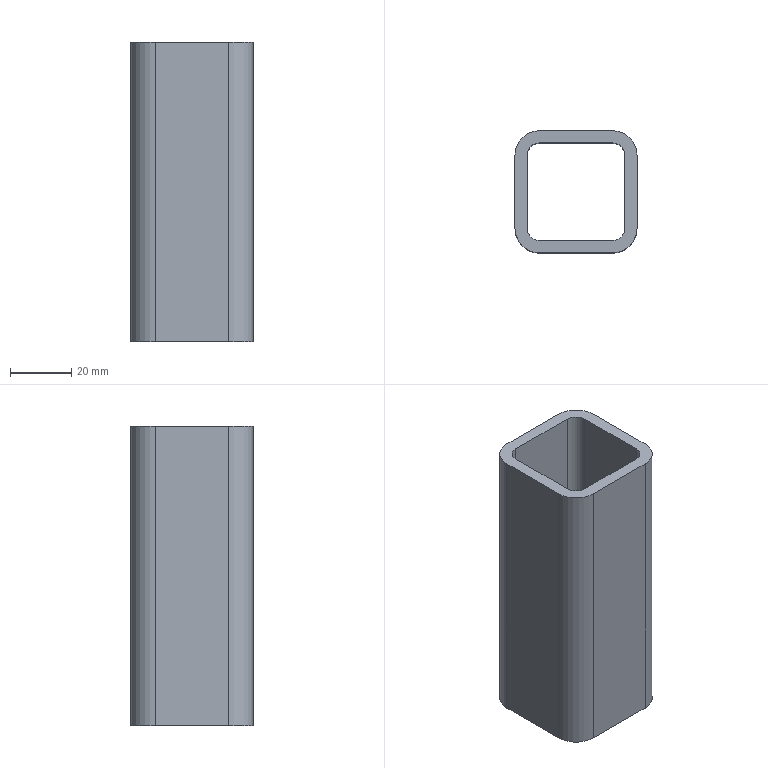Part | STEP file | 40 x 40 x 200 | 1 solid | 18 faces | box 40 x 40 x 98 mm | volume 52410 mm3 | plane 10 | cylinder 8 | commonest cylinder face diameters 8 x4 16 x4
STEP:
#1=CARTESIAN_POINT('',(36.,32.,-502.));
#2=VERTEX_POINT('',#1);
#3=CARTESIAN_POINT('',(32.,36.,-502.));
#4=VERTEX_POINT('',#3);
#5=CARTESIAN_POINT('',(32.,32.,-502.));
#6=DIRECTION('',(0.,0.,1.));
#7=DIRECTION('',(1.,0.,0.));
#8=AXIS2_PLACEMENT_3D('',#5,#6,#7);
#9=CIRCLE('',#8,4.);
#10=EDGE_CURVE('',#2,#4,#9,.T.);
#11=ORIENTED_EDGE('',*,*,#10,.T.);
#12=CARTESIAN_POINT('',(32.,36.,-600.));
#13=VERTEX_POINT('',#12);
#14=CARTESIAN_POINT('',(32.,36.,600.));
#15=DIRECTION('',(0.,0.,1.));
#16=VECTOR('',#15,1000.);
#17=LINE('',#14,#16);
#18=EDGE_CURVE('',#13,#4,#17,.T.);
#19=ORIENTED_EDGE('',*,*,#18,.F.);
#20=CARTESIAN_POINT('',(36.,32.,-600.));
#21=VERTEX_POINT('',#20);
#22=CARTESIAN_POINT('',(32.,32.,-600.));
#23=DIRECTION('',(0.,0.,-1.));
#24=DIRECTION('',(-1.,0.,0.));
#25=AXIS2_PLACEMENT_3D('',#22,#23,#24);
#26=CIRCLE('',#25,4.);
#27=EDGE_CURVE('',#13,#21,#26,.T.);
#28=ORIENTED_EDGE('',*,*,#27,.T.);
#29=CARTESIAN_POINT('',(36.,32.,600.));
#30=DIRECTION('',(0.,0.,-1.));
#31=VECTOR('',#30,1000.);
#32=LINE('',#29,#31);
#33=EDGE_CURVE('',#2,#21,#32,.T.);
#34=ORIENTED_EDGE('',*,*,#33,.F.);
#35=EDGE_LOOP('',(#11,#19,#28,#34));
#36=FACE_OUTER_BOUND('',#35,.T.);
#37=CARTESIAN_POINT('',(32.,32.,600.));
#38=DIRECTION('',(0.,0.,-1.));
#39=DIRECTION('',(-1.,0.,0.));
#40=AXIS2_PLACEMENT_3D('',#37,#38,#39);
#41=CYLINDRICAL_SURFACE('',#40,4.);
#42=ADVANCED_FACE('',(#36),#41,.F.);
#43=CARTESIAN_POINT('',(36.,8.,-600.));
#44=VERTEX_POINT('',#43);
#45=CARTESIAN_POINT('',(36.,8.,-502.));
#46=VERTEX_POINT('',#45);
#47=CARTESIAN_POINT('',(36.,8.,600.));
#48=DIRECTION('',(0.,0.,1.));
#49=VECTOR('',#48,1000.);
#50=LINE('',#47,#49);
#51=EDGE_CURVE('',#44,#46,#50,.T.);
#52=ORIENTED_EDGE('',*,*,#51,.T.);
#53=CARTESIAN_POINT('',(36.,32.,-502.));
#54=DIRECTION('',(0.,1.,0.));
#55=VECTOR('',#54,1000.);
#56=LINE('',#53,#55);
#57=EDGE_CURVE('',#46,#2,#56,.T.);
#58=ORIENTED_EDGE('',*,*,#57,.T.);
#59=ORIENTED_EDGE('',*,*,#33,.T.);
#60=CARTESIAN_POINT('',(36.,32.,-600.));
#61=DIRECTION('',(0.,-1.,0.));
#62=VECTOR('',#61,1000.);
#63=LINE('',#60,#62);
#64=EDGE_CURVE('',#21,#44,#63,.T.);
#65=ORIENTED_EDGE('',*,*,#64,.T.);
#66=EDGE_LOOP('',(#52,#58,#59,#65));
#67=FACE_OUTER_BOUND('',#66,.T.);
#68=CARTESIAN_POINT('',(36.,32.,600.));
#69=DIRECTION('',(-1.,0.,0.));
#70=DIRECTION('',(0.,0.,1.));
#71=AXIS2_PLACEMENT_3D('',#68,#69,#70);
#72=PLANE('',#71);
#73=ADVANCED_FACE('',(#67),#72,.T.);
#74=CARTESIAN_POINT('',(32.,4.,-502.));
#75=VERTEX_POINT('',#74);
#76=CARTESIAN_POINT('',(32.,8.,-502.));
#77=DIRECTION('',(0.,0.,1.));
#78=DIRECTION('',(1.,0.,0.));
#79=AXIS2_PLACEMENT_3D('',#76,#77,#78);
#80=CIRCLE('',#79,4.);
#81=EDGE_CURVE('',#75,#46,#80,.T.);
#82=ORIENTED_EDGE('',*,*,#81,.T.);
#83=ORIENTED_EDGE('',*,*,#51,.F.);
#84=CARTESIAN_POINT('',(32.,4.,-600.));
#85=VERTEX_POINT('',#84);
#86=CARTESIAN_POINT('',(32.,8.,-600.));
#87=DIRECTION('',(0.,0.,-1.));
#88=DIRECTION('',(-1.,0.,0.));
#89=AXIS2_PLACEMENT_3D('',#86,#87,#88);
#90=CIRCLE('',#89,4.);
#91=EDGE_CURVE('',#44,#85,#90,.T.);
#92=ORIENTED_EDGE('',*,*,#91,.T.);
#93=CARTESIAN_POINT('',(32.,4.,600.));
#94=DIRECTION('',(0.,0.,-1.));
#95=VECTOR('',#94,1000.);
#96=LINE('',#93,#95);
#97=EDGE_CURVE('',#75,#85,#96,.T.);
#98=ORIENTED_EDGE('',*,*,#97,.F.);
#99=EDGE_LOOP('',(#82,#83,#92,#98));
#100=FACE_OUTER_BOUND('',#99,.T.);
#101=CARTESIAN_POINT('',(32.,8.,600.));
#102=DIRECTION('',(0.,0.,-1.));
#103=DIRECTION('',(-1.,0.,0.));
#104=AXIS2_PLACEMENT_3D('',#101,#102,#103);
#105=CYLINDRICAL_SURFACE('',#104,4.);
#106=ADVANCED_FACE('',(#100),#105,.F.);
#107=CARTESIAN_POINT('',(8.,4.,-600.));
#108=VERTEX_POINT('',#107);
#109=CARTESIAN_POINT('',(8.,4.,-502.));
#110=VERTEX_POINT('',#109);
#111=CARTESIAN_POINT('',(8.,4.,600.));
#112=DIRECTION('',(0.,0.,1.));
#113=VECTOR('',#112,1000.);
#114=LINE('',#111,#113);
#115=EDGE_CURVE('',#108,#110,#114,.T.);
#116=ORIENTED_EDGE('',*,*,#115,.T.);
#117=CARTESIAN_POINT('',(32.,4.,-502.));
#118=DIRECTION('',(1.,0.,0.));
#119=VECTOR('',#118,1000.);
#120=LINE('',#117,#119);
#121=EDGE_CURVE('',#110,#75,#120,.T.);
#122=ORIENTED_EDGE('',*,*,#121,.T.);
#123=ORIENTED_EDGE('',*,*,#97,.T.);
#124=CARTESIAN_POINT('',(32.,4.,-600.));
#125=DIRECTION('',(-1.,0.,0.));
#126=VECTOR('',#125,1000.);
#127=LINE('',#124,#126);
#128=EDGE_CURVE('',#85,#108,#127,.T.);
#129=ORIENTED_EDGE('',*,*,#128,.T.);
#130=EDGE_LOOP('',(#116,#122,#123,#129));
#131=FACE_OUTER_BOUND('',#130,.T.);
#132=CARTESIAN_POINT('',(8.,4.,600.));
#133=DIRECTION('',(0.,1.,0.));
#134=DIRECTION('',(-1.,0.,0.));
#135=AXIS2_PLACEMENT_3D('',#132,#133,#134);
#136=PLANE('',#135);
#137=ADVANCED_FACE('',(#131),#136,.T.);
#138=CARTESIAN_POINT('',(4.,8.,-502.));
#139=VERTEX_POINT('',#138);
#140=CARTESIAN_POINT('',(8.,8.,-502.));
#141=DIRECTION('',(0.,0.,1.));
#142=DIRECTION('',(1.,0.,0.));
#143=AXIS2_PLACEMENT_3D('',#140,#141,#142);
#144=CIRCLE('',#143,4.);
#145=EDGE_CURVE('',#139,#110,#144,.T.);
#146=ORIENTED_EDGE('',*,*,#145,.T.);
#147=ORIENTED_EDGE('',*,*,#115,.F.);
#148=CARTESIAN_POINT('',(4.,8.,-600.));
#149=VERTEX_POINT('',#148);
#150=CARTESIAN_POINT('',(8.,8.,-600.));
#151=DIRECTION('',(0.,0.,-1.));
#152=DIRECTION('',(-1.,0.,0.));
#153=AXIS2_PLACEMENT_3D('',#150,#151,#152);
#154=CIRCLE('',#153,4.);
#155=EDGE_CURVE('',#108,#149,#154,.T.);
#156=ORIENTED_EDGE('',*,*,#155,.T.);
#157=CARTESIAN_POINT('',(4.,8.,600.));
#158=DIRECTION('',(0.,0.,-1.));
#159=VECTOR('',#158,1000.);
#160=LINE('',#157,#159);
#161=EDGE_CURVE('',#139,#149,#160,.T.);
#162=ORIENTED_EDGE('',*,*,#161,.F.);
#163=EDGE_LOOP('',(#146,#147,#156,#162));
#164=FACE_OUTER_BOUND('',#163,.T.);
#165=CARTESIAN_POINT('',(8.,8.,600.));
#166=DIRECTION('',(0.,0.,-1.));
#167=DIRECTION('',(-1.,0.,0.));
#168=AXIS2_PLACEMENT_3D('',#165,#166,#167);
#169=CYLINDRICAL_SURFACE('',#168,4.);
#170=ADVANCED_FACE('',(#164),#169,.F.);
#171=CARTESIAN_POINT('',(4.,32.,-600.));
#172=VERTEX_POINT('',#171);
#173=CARTESIAN_POINT('',(4.,32.,-502.));
#174=VERTEX_POINT('',#173);
#175=CARTESIAN_POINT('',(4.,32.,600.));
#176=DIRECTION('',(0.,0.,1.));
#177=VECTOR('',#176,1000.);
#178=LINE('',#175,#177);
#179=EDGE_CURVE('',#172,#174,#178,.T.);
#180=ORIENTED_EDGE('',*,*,#179,.T.);
#181=CARTESIAN_POINT('',(4.,8.,-502.));
#182=DIRECTION('',(0.,-1.,0.));
#183=VECTOR('',#182,1000.);
#184=LINE('',#181,#183);
#185=EDGE_CURVE('',#174,#139,#184,.T.);
#186=ORIENTED_EDGE('',*,*,#185,.T.);
#187=ORIENTED_EDGE('',*,*,#161,.T.);
#188=CARTESIAN_POINT('',(4.,32.,-600.));
#189=DIRECTION('',(0.,1.,0.));
#190=VECTOR('',#189,1000.);
#191=LINE('',#188,#190);
#192=EDGE_CURVE('',#149,#172,#191,.T.);
#193=ORIENTED_EDGE('',*,*,#192,.T.);
#194=EDGE_LOOP('',(#180,#186,#187,#193));
#195=FACE_OUTER_BOUND('',#194,.T.);
#196=CARTESIAN_POINT('',(4.,8.,600.));
#197=DIRECTION('',(1.,0.,0.));
#198=DIRECTION('',(0.,1.,0.));
#199=AXIS2_PLACEMENT_3D('',#196,#197,#198);
#200=PLANE('',#199);
#201=ADVANCED_FACE('',(#195),#200,.T.);
#202=CARTESIAN_POINT('',(8.,36.,-502.));
#203=VERTEX_POINT('',#202);
#204=CARTESIAN_POINT('',(8.,32.,-502.));
#205=DIRECTION('',(0.,0.,1.));
#206=DIRECTION('',(1.,0.,0.));
#207=AXIS2_PLACEMENT_3D('',#204,#205,#206);
#208=CIRCLE('',#207,4.);
#209=EDGE_CURVE('',#203,#174,#208,.T.);
#210=ORIENTED_EDGE('',*,*,#209,.T.);
#211=ORIENTED_EDGE('',*,*,#179,.F.);
#212=CARTESIAN_POINT('',(8.,36.,-600.));
#213=VERTEX_POINT('',#212);
#214=CARTESIAN_POINT('',(8.,32.,-600.));
#215=DIRECTION('',(0.,0.,-1.));
#216=DIRECTION('',(-1.,0.,0.));
#217=AXIS2_PLACEMENT_3D('',#214,#215,#216);
#218=CIRCLE('',#217,4.);
#219=EDGE_CURVE('',#172,#213,#218,.T.);
#220=ORIENTED_EDGE('',*,*,#219,.T.);
#221=CARTESIAN_POINT('',(8.,36.,600.));
#222=DIRECTION('',(0.,0.,-1.));
#223=VECTOR('',#222,1000.);
#224=LINE('',#221,#223);
#225=EDGE_CURVE('',#203,#213,#224,.T.);
#226=ORIENTED_EDGE('',*,*,#225,.F.);
#227=EDGE_LOOP('',(#210,#211,#220,#226));
#228=FACE_OUTER_BOUND('',#227,.T.);
#229=CARTESIAN_POINT('',(8.,32.,600.));
#230=DIRECTION('',(0.,0.,-1.));
#231=DIRECTION('',(-1.,0.,0.));
#232=AXIS2_PLACEMENT_3D('',#229,#230,#231);
#233=CYLINDRICAL_SURFACE('',#232,4.);
#234=ADVANCED_FACE('',(#228),#233,.F.);
#235=ORIENTED_EDGE('',*,*,#18,.T.);
#236=CARTESIAN_POINT('',(8.,36.,-502.));
#237=DIRECTION('',(-1.,0.,0.));
#238=VECTOR('',#237,1000.);
#239=LINE('',#236,#238);
#240=EDGE_CURVE('',#4,#203,#239,.T.);
#241=ORIENTED_EDGE('',*,*,#240,.T.);
#242=ORIENTED_EDGE('',*,*,#225,.T.);
#243=CARTESIAN_POINT('',(32.,36.,-600.));
#244=DIRECTION('',(1.,0.,0.));
#245=VECTOR('',#244,1000.);
#246=LINE('',#243,#245);
#247=EDGE_CURVE('',#213,#13,#246,.T.);
#248=ORIENTED_EDGE('',*,*,#247,.T.);
#249=EDGE_LOOP('',(#235,#241,#242,#248));
#250=FACE_OUTER_BOUND('',#249,.T.);
#251=CARTESIAN_POINT('',(32.,36.,600.));
#252=DIRECTION('',(0.,-1.,0.));
#253=DIRECTION('',(0.,0.,-1.));
#254=AXIS2_PLACEMENT_3D('',#251,#252,#253);
#255=PLANE('',#254);
#256=ADVANCED_FACE('',(#250),#255,.T.);
#257=CARTESIAN_POINT('',(40.,8.,-600.));
#258=VERTEX_POINT('',#257);
#259=CARTESIAN_POINT('',(40.,8.,-502.));
#260=VERTEX_POINT('',#259);
#261=CARTESIAN_POINT('',(40.,8.,600.));
#262=DIRECTION('',(0.,0.,1.));
#263=VECTOR('',#262,1000.);
#264=LINE('',#261,#263);
#265=EDGE_CURVE('',#258,#260,#264,.T.);
#266=ORIENTED_EDGE('',*,*,#265,.T.);
#267=CARTESIAN_POINT('',(32.,0.,-502.));
#268=VERTEX_POINT('',#267);
#269=CARTESIAN_POINT('',(32.,8.,-502.));
#270=DIRECTION('',(0.,0.,1.));
#271=DIRECTION('',(1.,0.,0.));
#272=AXIS2_PLACEMENT_3D('',#269,#270,#271);
#273=CIRCLE('',#272,8.);
#274=EDGE_CURVE('',#268,#260,#273,.T.);
#275=ORIENTED_EDGE('',*,*,#274,.F.);
#276=CARTESIAN_POINT('',(32.,0.,-600.));
#277=VERTEX_POINT('',#276);
#278=CARTESIAN_POINT('',(32.,0.,600.));
#279=DIRECTION('',(0.,0.,-1.));
#280=VECTOR('',#279,1000.);
#281=LINE('',#278,#280);
#282=EDGE_CURVE('',#268,#277,#281,.T.);
#283=ORIENTED_EDGE('',*,*,#282,.T.);
#284=CARTESIAN_POINT('',(32.,8.,-600.));
#285=DIRECTION('',(0.,0.,1.));
#286=DIRECTION('',(-1.,0.,0.));
#287=AXIS2_PLACEMENT_3D('',#284,#285,#286);
#288=CIRCLE('',#287,8.);
#289=EDGE_CURVE('',#277,#258,#288,.T.);
#290=ORIENTED_EDGE('',*,*,#289,.T.);
#291=EDGE_LOOP('',(#266,#275,#283,#290));
#292=FACE_OUTER_BOUND('',#291,.T.);
#293=CARTESIAN_POINT('',(32.,8.,600.));
#294=DIRECTION('',(0.,0.,-1.));
#295=DIRECTION('',(-1.,0.,0.));
#296=AXIS2_PLACEMENT_3D('',#293,#294,#295);
#297=CYLINDRICAL_SURFACE('',#296,8.);
#298=ADVANCED_FACE('',(#292),#297,.T.);
#299=CARTESIAN_POINT('',(40.,32.,-502.));
#300=VERTEX_POINT('',#299);
#301=CARTESIAN_POINT('',(40.,8.,-502.));
#302=DIRECTION('',(0.,1.,0.));
#303=VECTOR('',#302,1000.);
#304=LINE('',#301,#303);
#305=EDGE_CURVE('',#260,#300,#304,.T.);
#306=ORIENTED_EDGE('',*,*,#305,.F.);
#307=ORIENTED_EDGE('',*,*,#265,.F.);
#308=CARTESIAN_POINT('',(40.,32.,-600.));
#309=VERTEX_POINT('',#308);
#310=CARTESIAN_POINT('',(40.,32.,-600.));
#311=DIRECTION('',(0.,1.,0.));
#312=VECTOR('',#311,1000.);
#313=LINE('',#310,#312);
#314=EDGE_CURVE('',#258,#309,#313,.T.);
#315=ORIENTED_EDGE('',*,*,#314,.T.);
#316=CARTESIAN_POINT('',(40.,32.,600.));
#317=DIRECTION('',(0.,0.,-1.));
#318=VECTOR('',#317,1000.);
#319=LINE('',#316,#318);
#320=EDGE_CURVE('',#300,#309,#319,.T.);
#321=ORIENTED_EDGE('',*,*,#320,.F.);
#322=EDGE_LOOP('',(#306,#307,#315,#321));
#323=FACE_OUTER_BOUND('',#322,.T.);
#324=CARTESIAN_POINT('',(40.,32.,600.));
#325=DIRECTION('',(-1.,0.,0.));
#326=DIRECTION('',(0.,-1.,0.));
#327=AXIS2_PLACEMENT_3D('',#324,#325,#326);
#328=PLANE('',#327);
#329=ADVANCED_FACE('',(#323),#328,.F.);
#330=CARTESIAN_POINT('',(32.,40.,-600.));
#331=VERTEX_POINT('',#330);
#332=CARTESIAN_POINT('',(32.,40.,-502.));
#333=VERTEX_POINT('',#332);
#334=CARTESIAN_POINT('',(32.,40.,600.));
#335=DIRECTION('',(0.,0.,1.));
#336=VECTOR('',#335,1000.);
#337=LINE('',#334,#336);
#338=EDGE_CURVE('',#331,#333,#337,.T.);
#339=ORIENTED_EDGE('',*,*,#338,.T.);
#340=CARTESIAN_POINT('',(32.,32.,-502.));
#341=DIRECTION('',(0.,0.,1.));
#342=DIRECTION('',(1.,0.,0.));
#343=AXIS2_PLACEMENT_3D('',#340,#341,#342);
#344=CIRCLE('',#343,8.);
#345=EDGE_CURVE('',#300,#333,#344,.T.);
#346=ORIENTED_EDGE('',*,*,#345,.F.);
#347=ORIENTED_EDGE('',*,*,#320,.T.);
#348=CARTESIAN_POINT('',(32.,32.,-600.));
#349=DIRECTION('',(0.,0.,1.));
#350=DIRECTION('',(-1.,0.,0.));
#351=AXIS2_PLACEMENT_3D('',#348,#349,#350);
#352=CIRCLE('',#351,8.);
#353=EDGE_CURVE('',#309,#331,#352,.T.);
#354=ORIENTED_EDGE('',*,*,#353,.T.);
#355=EDGE_LOOP('',(#339,#346,#347,#354));
#356=FACE_OUTER_BOUND('',#355,.T.);
#357=CARTESIAN_POINT('',(32.,32.,600.));
#358=DIRECTION('',(0.,0.,-1.));
#359=DIRECTION('',(-1.,0.,0.));
#360=AXIS2_PLACEMENT_3D('',#357,#358,#359);
#361=CYLINDRICAL_SURFACE('',#360,8.);
#362=ADVANCED_FACE('',(#356),#361,.T.);
#363=CARTESIAN_POINT('',(8.,40.,-502.));
#364=VERTEX_POINT('',#363);
#365=CARTESIAN_POINT('',(32.,40.,-502.));
#366=DIRECTION('',(-1.,0.,0.));
#367=VECTOR('',#366,1000.);
#368=LINE('',#365,#367);
#369=EDGE_CURVE('',#333,#364,#368,.T.);
#370=ORIENTED_EDGE('',*,*,#369,.F.);
#371=ORIENTED_EDGE('',*,*,#338,.F.);
#372=CARTESIAN_POINT('',(8.,40.,-600.));
#373=VERTEX_POINT('',#372);
#374=CARTESIAN_POINT('',(32.,40.,-600.));
#375=DIRECTION('',(-1.,0.,0.));
#376=VECTOR('',#375,1000.);
#377=LINE('',#374,#376);
#378=EDGE_CURVE('',#331,#373,#377,.T.);
#379=ORIENTED_EDGE('',*,*,#378,.T.);
#380=CARTESIAN_POINT('',(8.,40.,600.));
#381=DIRECTION('',(0.,0.,-1.));
#382=VECTOR('',#381,1000.);
#383=LINE('',#380,#382);
#384=EDGE_CURVE('',#364,#373,#383,.T.);
#385=ORIENTED_EDGE('',*,*,#384,.F.);
#386=EDGE_LOOP('',(#370,#371,#379,#385));
#387=FACE_OUTER_BOUND('',#386,.T.);
#388=CARTESIAN_POINT('',(32.,40.,600.));
#389=DIRECTION('',(0.,-1.,0.));
#390=DIRECTION('',(1.,0.,0.));
#391=AXIS2_PLACEMENT_3D('',#388,#389,#390);
#392=PLANE('',#391);
#393=ADVANCED_FACE('',(#387),#392,.F.);
#394=CARTESIAN_POINT('',(8.,0.,-502.));
#395=VERTEX_POINT('',#394);
#396=CARTESIAN_POINT('',(8.,0.,-502.));
#397=DIRECTION('',(1.,0.,0.));
#398=VECTOR('',#397,1000.);
#399=LINE('',#396,#398);
#400=EDGE_CURVE('',#395,#268,#399,.T.);
#401=ORIENTED_EDGE('',*,*,#400,.F.);
#402=CARTESIAN_POINT('',(8.,0.,-600.));
#403=VERTEX_POINT('',#402);
#404=CARTESIAN_POINT('',(8.,0.,600.));
#405=DIRECTION('',(0.,0.,1.));
#406=VECTOR('',#405,1000.);
#407=LINE('',#404,#406);
#408=EDGE_CURVE('',#403,#395,#407,.T.);
#409=ORIENTED_EDGE('',*,*,#408,.F.);
#410=CARTESIAN_POINT('',(32.,0.,-600.));
#411=DIRECTION('',(1.,0.,0.));
#412=VECTOR('',#411,1000.);
#413=LINE('',#410,#412);
#414=EDGE_CURVE('',#403,#277,#413,.T.);
#415=ORIENTED_EDGE('',*,*,#414,.T.);
#416=ORIENTED_EDGE('',*,*,#282,.F.);
#417=EDGE_LOOP('',(#401,#409,#415,#416));
#418=FACE_OUTER_BOUND('',#417,.T.);
#419=CARTESIAN_POINT('',(8.,0.,600.));
#420=DIRECTION('',(0.,1.,0.));
#421=DIRECTION('',(-1.,0.,0.));
#422=AXIS2_PLACEMENT_3D('',#419,#420,#421);
#423=PLANE('',#422);
#424=ADVANCED_FACE('',(#418),#423,.F.);
#425=ORIENTED_EDGE('',*,*,#408,.T.);
#426=CARTESIAN_POINT('',(0.,8.,-502.));
#427=VERTEX_POINT('',#426);
#428=CARTESIAN_POINT('',(8.,8.,-502.));
#429=DIRECTION('',(0.,0.,1.));
#430=DIRECTION('',(1.,0.,0.));
#431=AXIS2_PLACEMENT_3D('',#428,#429,#430);
#432=CIRCLE('',#431,8.);
#433=EDGE_CURVE('',#427,#395,#432,.T.);
#434=ORIENTED_EDGE('',*,*,#433,.F.);
#435=CARTESIAN_POINT('',(0.,8.,-600.));
#436=VERTEX_POINT('',#435);
#437=CARTESIAN_POINT('',(0.,8.,600.));
#438=DIRECTION('',(0.,0.,-1.));
#439=VECTOR('',#438,1000.);
#440=LINE('',#437,#439);
#441=EDGE_CURVE('',#427,#436,#440,.T.);
#442=ORIENTED_EDGE('',*,*,#441,.T.);
#443=CARTESIAN_POINT('',(8.,8.,-600.));
#444=DIRECTION('',(0.,0.,1.));
#445=DIRECTION('',(-1.,0.,0.));
#446=AXIS2_PLACEMENT_3D('',#443,#444,#445);
#447=CIRCLE('',#446,8.);
#448=EDGE_CURVE('',#436,#403,#447,.T.);
#449=ORIENTED_EDGE('',*,*,#448,.T.);
#450=EDGE_LOOP('',(#425,#434,#442,#449));
#451=FACE_OUTER_BOUND('',#450,.T.);
#452=CARTESIAN_POINT('',(8.,8.,600.));
#453=DIRECTION('',(0.,0.,-1.));
#454=DIRECTION('',(-1.,0.,0.));
#455=AXIS2_PLACEMENT_3D('',#452,#453,#454);
#456=CYLINDRICAL_SURFACE('',#455,8.);
#457=ADVANCED_FACE('',(#451),#456,.T.);
#458=CARTESIAN_POINT('',(0.,32.,-600.));
#459=VERTEX_POINT('',#458);
#460=CARTESIAN_POINT('',(0.,32.,-502.));
#461=VERTEX_POINT('',#460);
#462=CARTESIAN_POINT('',(0.,32.,600.));
#463=DIRECTION('',(0.,0.,1.));
#464=VECTOR('',#463,1000.);
#465=LINE('',#462,#464);
#466=EDGE_CURVE('',#459,#461,#465,.T.);
#467=ORIENTED_EDGE('',*,*,#466,.T.);
#468=CARTESIAN_POINT('',(8.,32.,-502.));
#469=DIRECTION('',(0.,0.,1.));
#470=DIRECTION('',(1.,0.,0.));
#471=AXIS2_PLACEMENT_3D('',#468,#469,#470);
#472=CIRCLE('',#471,8.);
#473=EDGE_CURVE('',#364,#461,#472,.T.);
#474=ORIENTED_EDGE('',*,*,#473,.F.);
#475=ORIENTED_EDGE('',*,*,#384,.T.);
#476=CARTESIAN_POINT('',(8.,32.,-600.));
#477=DIRECTION('',(0.,0.,1.));
#478=DIRECTION('',(-1.,0.,0.));
#479=AXIS2_PLACEMENT_3D('',#476,#477,#478);
#480=CIRCLE('',#479,8.);
#481=EDGE_CURVE('',#373,#459,#480,.T.);
#482=ORIENTED_EDGE('',*,*,#481,.T.);
#483=EDGE_LOOP('',(#467,#474,#475,#482));
#484=FACE_OUTER_BOUND('',#483,.T.);
#485=CARTESIAN_POINT('',(8.,32.,600.));
#486=DIRECTION('',(0.,0.,-1.));
#487=DIRECTION('',(-1.,0.,0.));
#488=AXIS2_PLACEMENT_3D('',#485,#486,#487);
#489=CYLINDRICAL_SURFACE('',#488,8.);
#490=ADVANCED_FACE('',(#484),#489,.T.);
#491=CARTESIAN_POINT('',(0.,32.,-502.));
#492=DIRECTION('',(0.,-1.,0.));
#493=VECTOR('',#492,1000.);
#494=LINE('',#491,#493);
#495=EDGE_CURVE('',#461,#427,#494,.T.);
#496=ORIENTED_EDGE('',*,*,#495,.F.);
#497=ORIENTED_EDGE('',*,*,#466,.F.);
#498=CARTESIAN_POINT('',(0.,8.,-600.));
#499=DIRECTION('',(0.,1.,0.));
#500=VECTOR('',#499,1000.);
#501=LINE('',#498,#500);
#502=EDGE_CURVE('',#436,#459,#501,.T.);
#503=ORIENTED_EDGE('',*,*,#502,.F.);
#504=ORIENTED_EDGE('',*,*,#441,.F.);
#505=EDGE_LOOP('',(#496,#497,#503,#504));
#506=FACE_OUTER_BOUND('',#505,.T.);
#507=CARTESIAN_POINT('',(0.,8.,600.));
#508=DIRECTION('',(1.,0.,0.));
#509=DIRECTION('',(0.,1.,0.));
#510=AXIS2_PLACEMENT_3D('',#507,#508,#509);
#511=PLANE('',#510);
#512=ADVANCED_FACE('',(#506),#511,.F.);
#513=ORIENTED_EDGE('',*,*,#289,.F.);
#514=ORIENTED_EDGE('',*,*,#414,.F.);
#515=ORIENTED_EDGE('',*,*,#448,.F.);
#516=ORIENTED_EDGE('',*,*,#502,.T.);
#517=ORIENTED_EDGE('',*,*,#481,.F.);
#518=ORIENTED_EDGE('',*,*,#378,.F.);
#519=ORIENTED_EDGE('',*,*,#353,.F.);
#520=ORIENTED_EDGE('',*,*,#314,.F.);
#521=EDGE_LOOP('',(#513,#514,#515,#516,#517,#518,#519,#520));
#522=FACE_OUTER_BOUND('',#521,.T.);
#523=ORIENTED_EDGE('',*,*,#155,.F.);
#524=ORIENTED_EDGE('',*,*,#128,.F.);
#525=ORIENTED_EDGE('',*,*,#91,.F.);
#526=ORIENTED_EDGE('',*,*,#64,.F.);
#527=ORIENTED_EDGE('',*,*,#27,.F.);
#528=ORIENTED_EDGE('',*,*,#247,.F.);
#529=ORIENTED_EDGE('',*,*,#219,.F.);
#530=ORIENTED_EDGE('',*,*,#192,.F.);
#531=EDGE_LOOP('',(#523,#524,#525,#526,#527,#528,#529,#530));
#532=FACE_BOUND('',#531,.T.);
#533=CARTESIAN_POINT('',(32.,32.,-600.));
#534=DIRECTION('',(0.,0.,1.));
#535=DIRECTION('',(1.,0.,0.));
#536=AXIS2_PLACEMENT_3D('',#533,#534,#535);
#537=PLANE('',#536);
#538=ADVANCED_FACE('',(#522,#532),#537,.F.);
#539=ORIENTED_EDGE('',*,*,#57,.F.);
#540=ORIENTED_EDGE('',*,*,#81,.F.);
#541=ORIENTED_EDGE('',*,*,#121,.F.);
#542=ORIENTED_EDGE('',*,*,#145,.F.);
#543=ORIENTED_EDGE('',*,*,#185,.F.);
#544=ORIENTED_EDGE('',*,*,#209,.F.);
#545=ORIENTED_EDGE('',*,*,#240,.F.);
#546=ORIENTED_EDGE('',*,*,#10,.F.);
#547=EDGE_LOOP('',(#539,#540,#541,#542,#543,#544,#545,#546));
#548=FACE_BOUND('',#547,.T.);
#549=ORIENTED_EDGE('',*,*,#433,.T.);
#550=ORIENTED_EDGE('',*,*,#400,.T.);
#551=ORIENTED_EDGE('',*,*,#274,.T.);
#552=ORIENTED_EDGE('',*,*,#305,.T.);
#553=ORIENTED_EDGE('',*,*,#345,.T.);
#554=ORIENTED_EDGE('',*,*,#369,.T.);
#555=ORIENTED_EDGE('',*,*,#473,.T.);
#556=ORIENTED_EDGE('',*,*,#495,.T.);
#557=EDGE_LOOP('',(#549,#550,#551,#552,#553,#554,#555,#556));
#558=FACE_OUTER_BOUND('',#557,.T.);
#559=CARTESIAN_POINT('',(8.,8.,-502.));
#560=DIRECTION('',(0.,0.,1.));
#561=DIRECTION('',(1.,0.,0.));
#562=AXIS2_PLACEMENT_3D('',#559,#560,#561);
#563=PLANE('',#562);
#564=ADVANCED_FACE('',(#548,#558),#563,.T.);
#565=CLOSED_SHELL('',(#42,#73,#106,#137,#170,#201,#234,#256,#298,#329,#362,#393,#424,#457,#490,#512,#538,#564));
#566=MANIFOLD_SOLID_BREP('',#565);
#567=CARTESIAN_POINT('',(0.,0.,0.));
#568=DIRECTION('',(0.,0.,1.));
#569=DIRECTION('',(1.,0.,0.));
#570=AXIS2_PLACEMENT_3D('',#567,#568,#569);
#571=(LENGTH_UNIT()NAMED_UNIT(*)SI_UNIT(.MILLI.,.METRE.));
#572=UNCERTAINTY_MEASURE_WITH_UNIT(LENGTH_MEASURE(0.00001),#571,'','');
#573=(NAMED_UNIT(*)PLANE_ANGLE_UNIT()SI_UNIT($,.RADIAN.));
#574=(NAMED_UNIT(*)SI_UNIT($,.STERADIAN.)SOLID_ANGLE_UNIT());
#575=(GEOMETRIC_REPRESENTATION_CONTEXT(3)GLOBAL_UNCERTAINTY_ASSIGNED_CONTEXT((#572))GLOBAL_UNIT_ASSIGNED_CONTEXT((#571,#573,#574))REPRESENTATION_CONTEXT('',''));
#576=ADVANCED_BREP_SHAPE_REPRESENTATION('',(#566,#570),#575);